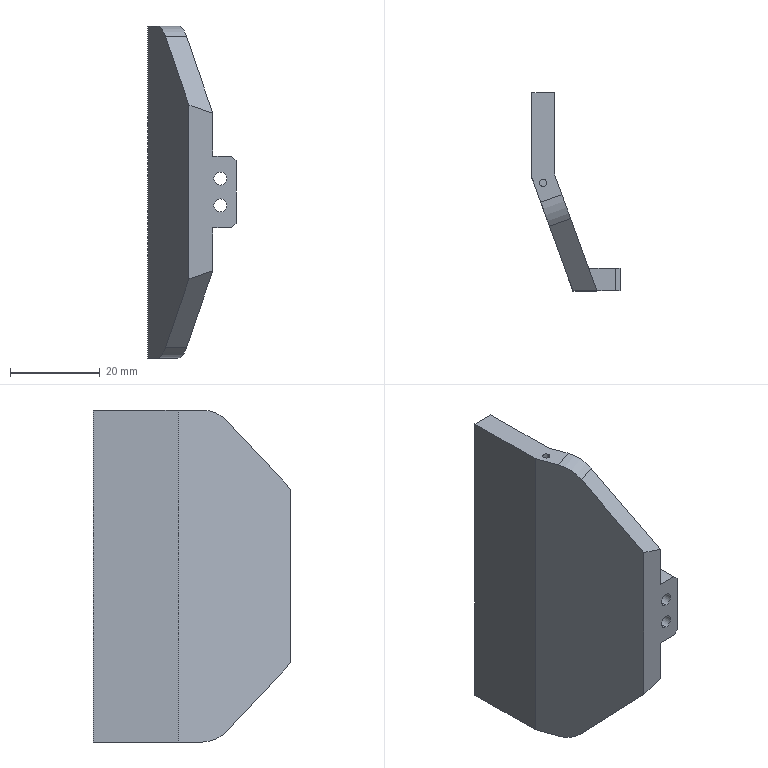NC program | NX | posted with a generic post | part box 19.643 x 44.061 x 74 mm
Whole program:
N10 G17 G21 G94 G90
(PLANAR_MILL_1 , TOOL : D3开粗)
N12 T11 M6
N14 G54
N16 G17 G0 G90 X40.536 Y-35.354 B0. C0. S4500 M3
N18 G43 Z30. H11
N20 Z2.7
N22 G94 G1 Z-0.3 F2000.
N24 X38.414 Y-37.475
N26 X37.414 Y-38.475
N28 G2 X36. Y-39.061 R2.
N30 G1 X32.
N32 G2 X30.586 Y-38.475 R2.
N34 G1 X29.586 Y-37.475
N36 X27.464 Y-35.354
N38 Z2.7
N40 G0 Z30.
N42 X40.536
N44 Z2.4
N46 G1 Z-0.6
N48 X38.414 Y-37.475
N50 X37.414 Y-38.475
N52 G2 X36. Y-39.061 R2.
N54 G1 X32.
N56 G2 X30.586 Y-38.475 R2.
N58 G1 X29.586 Y-37.475
N60 X27.464 Y-35.354
N62 Z2.4
N64 G0 Z30.
N66 X40.536
N68 Z2.1
N70 G1 Z-0.9
N72 X38.414 Y-37.475
N74 X37.414 Y-38.475
N76 G2 X36. Y-39.061 R2.
N78 G1 X32.
N80 G2 X30.586 Y-38.475 R2.
N82 G1 X29.586 Y-37.475
N84 X27.464 Y-35.354
N86 Z2.1
N88 G0 Z30.
N90 X40.536
N92 Z1.8
N94 G1 Z-1.2
N96 X38.414 Y-37.475
N98 X37.414 Y-38.475
N100 G2 X36. Y-39.061 R2.
N102 G1 X32.
N104 G2 X30.586 Y-38.475 R2.
N106 G1 X29.586 Y-37.475
N108 X27.464 Y-35.354
N110 Z1.8
N112 G0 Z30.
N114 X40.536
N116 Z1.5
N118 G1 Z-1.5
N120 X38.414 Y-37.475
N122 X37.414 Y-38.475
N124 G2 X36. Y-39.061 R2.
N126 G1 X32.
N128 G2 X30.586 Y-38.475 R2.
N130 G1 X29.586 Y-37.475
N132 X27.464 Y-35.354
N134 Z1.5
N136 G0 Z30.
N138 X40.536
N140 Z1.2
N142 G1 Z-1.8
N144 X38.414 Y-37.475
N146 X37.414 Y-38.475
N148 G2 X36. Y-39.061 R2.
N150 G1 X32.
N152 G2 X30.586 Y-38.475 R2.
N154 G1 X29.586 Y-37.475
N156 X27.464 Y-35.354
N158 Z1.2
N160 G0 Z30.
N162 X40.536
N164 Z0.9
N166 G1 Z-2.1
N168 X38.414 Y-37.475
N170 X37.414 Y-38.475
N172 G2 X36. Y-39.061 R2.
N174 G1 X32.
N176 G2 X30.586 Y-38.475 R2.
N178 G1 X29.586 Y-37.475
N180 X27.464 Y-35.354
N182 Z0.9
N184 G0 Z30.
N186 X40.536
N188 Z0.6
N190 G1 Z-2.4
N192 X38.414 Y-37.475
N194 X37.414 Y-38.475
N196 G2 X36. Y-39.061 R2.
N198 G1 X32.
N200 G2 X30.586 Y-38.475 R2.
N202 G1 X29.586 Y-37.475
N204 X27.464 Y-35.354
N206 Z0.6
N208 G0 Z30.
N210 X40.536
N212 Z0.3
N214 G1 Z-2.7
N216 X38.414 Y-37.475
N218 X37.414 Y-38.475
N220 G2 X36. Y-39.061 R2.
N222 G1 X32.
N224 G2 X30.586 Y-38.475 R2.
N226 G1 X29.586 Y-37.475
N228 X27.464 Y-35.354
N230 Z0.3
N232 G0 Z30.
N234 X40.536
N236 Z0.
N238 G1 Z-3.
N240 X38.414 Y-37.475
N242 X37.414 Y-38.475
N244 G2 X36. Y-39.061 R2.
N246 G1 X32.
N248 G2 X30.586 Y-38.475 R2.
N250 G1 X29.586 Y-37.475
N252 X27.464 Y-35.354
N254 Z0.
N256 G0 Z30.
N258 X40.536
N260 Z-0.3
N262 G1 Z-3.3
N264 X38.414 Y-37.475
N266 X37.414 Y-38.475
N268 G2 X36. Y-39.061 R2.
N270 G1 X32.
N272 G2 X30.586 Y-38.475 R2.
N274 G1 X29.586 Y-37.475
N276 X27.464 Y-35.354
N278 Z-0.3
N280 G0 Z30.
N282 X40.536
N284 Z-0.6
N286 G1 Z-3.6
N288 X38.414 Y-37.475
N290 X37.414 Y-38.475
N292 G2 X36. Y-39.061 R2.
N294 G1 X32.
N296 G2 X30.586 Y-38.475 R2.
N298 G1 X29.586 Y-37.475
N300 X27.464 Y-35.354
N302 Z-0.6
N304 G0 Z30.
N306 X40.536
N308 Z-0.9
N310 G1 Z-3.9
N312 X38.414 Y-37.475
N314 X37.414 Y-38.475
N316 G2 X36. Y-39.061 R2.
N318 G1 X32.
N320 G2 X30.586 Y-38.475 R2.
N322 G1 X29.586 Y-37.475
N324 X27.464 Y-35.354
N326 Z-0.9
N328 G0 Z30.
N330 X40.536
N332 Z-1.2
N334 G1 Z-4.2
N336 X38.414 Y-37.475
N338 X37.414 Y-38.475
N340 G2 X36. Y-39.061 R2.
N342 G1 X32.
N344 G2 X30.586 Y-38.475 R2.
N346 G1 X29.586 Y-37.475
N348 X27.464 Y-35.354
N350 Z-1.2
N352 G0 Z30.
N354 X40.536
N356 Z-1.5
N358 G1 Z-4.5
N360 X38.414 Y-37.475
N362 X37.414 Y-38.475
N364 G2 X36. Y-39.061 R2.
N366 G1 X32.
N368 G2 X30.586 Y-38.475 R2.
N370 G1 X29.586 Y-37.475
N372 X27.464 Y-35.354
N374 Z-1.5
N376 G0 Z30.
N378 X40.536
N380 Z-1.8
N382 G1 Z-4.8
N384 X38.414 Y-37.475
N386 X37.414 Y-38.475
N388 G2 X36. Y-39.061 R2.
N390 G1 X32.
N392 G2 X30.586 Y-38.475 R2.
N394 G1 X29.586 Y-37.475
N396 X27.464 Y-35.354
N398 Z-1.8
N400 G0 Z30.
N402 X-27.464
N404 Z2.7
N406 G1 Z-0.3
N408 X-29.586 Y-37.475
N410 X-30.586 Y-38.475
N412 G2 X-32. Y-39.061 R2.
N414 G1 X-36.
N416 G2 X-37.414 Y-38.475 R2.
N418 G1 X-38.414 Y-37.475
N420 X-40.536 Y-35.354
N422 Z2.7
N424 G0 Z30.
N426 X-27.464
N428 Z2.4
N430 G1 Z-0.6
N432 X-29.586 Y-37.475
N434 X-30.586 Y-38.475
N436 G2 X-32. Y-39.061 R2.
N438 G1 X-36.
N440 G2 X-37.414 Y-38.475 R2.
N442 G1 X-38.414 Y-37.475
N444 X-40.536 Y-35.354
N446 Z2.4
N448 G0 Z30.
N450 X-27.464
N452 Z2.1
N454 G1 Z-0.9
N456 X-29.586 Y-37.475
N458 X-30.586 Y-38.475
N460 G2 X-32. Y-39.061 R2.
N462 G1 X-36.
N464 G2 X-37.414 Y-38.475 R2.
N466 G1 X-38.414 Y-37.475
N468 X-40.536 Y-35.354
N470 Z2.1
N472 G0 Z30.
N474 X-27.464
N476 Z1.8
N478 G1 Z-1.2
N480 X-29.586 Y-37.475
N482 X-30.586 Y-38.475
N484 G2 X-32. Y-39.061 R2.
N486 G1 X-36.
N488 G2 X-37.414 Y-38.475 R2.
N490 G1 X-38.414 Y-37.475
N492 X-40.536 Y-35.354
N494 Z1.8
N496 G0 Z30.
N498 X-27.464
N500 Z1.5
N502 G1 Z-1.5
N504 X-29.586 Y-37.475
N506 X-30.586 Y-38.475
N508 G2 X-32. Y-39.061 R2.
N510 G1 X-36.
N512 G2 X-37.414 Y-38.475 R2.
N514 G1 X-38.414 Y-37.475
N516 X-40.536 Y-35.354
N518 Z1.5
N520 G0 Z30.
N522 X-27.464
N524 Z1.2
N526 G1 Z-1.8
N528 X-29.586 Y-37.475
N530 X-30.586 Y-38.475
N532 G2 X-32. Y-39.061 R2.
N534 G1 X-36.
N536 G2 X-37.414 Y-38.475 R2.
N538 G1 X-38.414 Y-37.475
N540 X-40.536 Y-35.354
N542 Z1.2
N544 G0 Z30.
N546 X-27.464
N548 Z0.9
N550 G1 Z-2.1
N552 X-29.586 Y-37.475
N554 X-30.586 Y-38.475
N556 G2 X-32. Y-39.061 R2.
N558 G1 X-36.
N560 G2 X-37.414 Y-38.475 R2.
N562 G1 X-38.414 Y-37.475
N564 X-40.536 Y-35.354
N566 Z0.9
N568 G0 Z30.
N570 X-27.464
N572 Z0.6
N574 G1 Z-2.4
N576 X-29.586 Y-37.475
N578 X-30.586 Y-38.475
N580 G2 X-32. Y-39.061 R2.
N582 G1 X-36.
N584 G2 X-37.414 Y-38.475 R2.
N586 G1 X-38.414 Y-37.475
N588 X-40.536 Y-35.354
N590 Z0.6
N592 G0 Z30.
N594 X-27.464
N596 Z0.3
N598 G1 Z-2.7
N600 X-29.586 Y-37.475
N602 X-30.586 Y-38.475
N604 G2 X-32. Y-39.061 R2.
N606 G1 X-36.
N608 G2 X-37.414 Y-38.475 R2.
N610 G1 X-38.414 Y-37.475
N612 X-40.536 Y-35.354
N614 Z0.3
N616 G0 Z30.
N618 X-27.464
N620 Z0.
N622 G1 Z-3.
N624 X-29.586 Y-37.475
N626 X-30.586 Y-38.475
N628 G2 X-32. Y-39.061 R2.
N630 G1 X-36.
N632 G2 X-37.414 Y-38.475 R2.
N634 G1 X-38.414 Y-37.475
N636 X-40.536 Y-35.354
N638 Z0.
N640 G0 Z30.
N642 X-27.464
N644 Z-0.3
N646 G1 Z-3.3
N648 X-29.586 Y-37.475
N650 X-30.586 Y-38.475
N652 G2 X-32. Y-39.061 R2.
N654 G1 X-36.
N656 G2 X-37.414 Y-38.475 R2.
N658 G1 X-38.414 Y-37.475
N660 X-40.536 Y-35.354
N662 Z-0.3
N664 G0 Z30.
N666 X-27.464
N668 Z-0.6
N670 G1 Z-3.6
N672 X-29.586 Y-37.475
N674 X-30.586 Y-38.475
N676 G2 X-32. Y-39.061 R2.
N678 G1 X-36.
N680 G2 X-37.414 Y-38.475 R2.
N682 G1 X-38.414 Y-37.475
N684 X-40.536 Y-35.354
N686 Z-0.6
N688 G0 Z30.
N690 X-27.464
N692 Z-0.9
N694 G1 Z-3.9
N696 X-29.586 Y-37.475
N698 X-30.586 Y-38.475
N700 G2 X-32. Y-39.061 R2.
N702 G1 X-36.
N704 G2 X-37.414 Y-38.475 R2.
N706 G1 X-38.414 Y-37.475
N708 X-40.536 Y-35.354
N710 Z-0.9
N712 G0 Z30.
N714 X-27.464
N716 Z-1.2
N718 G1 Z-4.2
N720 X-29.586 Y-37.475
N722 X-30.586 Y-38.475
N724 G2 X-32. Y-39.061 R2.
N726 G1 X-36.
N728 G2 X-37.414 Y-38.475 R2.
N730 G1 X-38.414 Y-37.475
N732 X-40.536 Y-35.354
N734 Z-1.2
N736 G0 Z30.
N738 X-27.464
N740 Z-1.5
N742 G1 Z-4.5
N744 X-29.586 Y-37.475
N746 X-30.586 Y-38.475
N748 G2 X-32. Y-39.061 R2.
N750 G1 X-36.
N752 G2 X-37.414 Y-38.475 R2.
N754 G1 X-38.414 Y-37.475
N756 X-40.536 Y-35.354
N758 Z-1.5
N760 G0 Z30.
N762 X-27.464
N764 Z-1.8
N766 G1 Z-4.8
N768 X-29.586 Y-37.475
N770 X-30.586 Y-38.475
N772 G2 X-32. Y-39.061 R2.
N774 G1 X-36.
N776 G2 X-37.414 Y-38.475 R2.
N778 G1 X-38.414 Y-37.475
N780 X-40.536 Y-35.354
N782 Z-1.8
N784 G0 Z30.
N786 M5
N788 M2